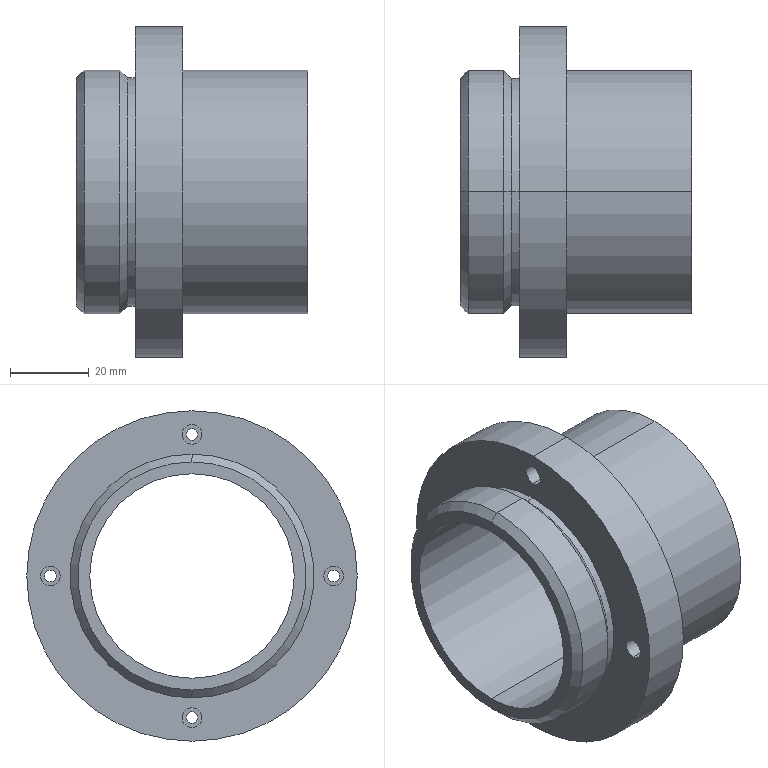Part | SolidWorks | features Chamfer 2, ICE 2, Revolution 1 | 1 solid | 38 faces | box 58.8 x 84 x 84 mm | volume 80812 mm3 | cylinder 26 | plane 8 | cone 4 | commonest cylinder face diameters 3 x8 5 x8 62 x4 52 x2 58 x2 84 x2
STEP:
#1=CARTESIAN_POINT('',(-17.378,0.,33.5));
#2=VERTEX_POINT('',#1);
#3=CARTESIAN_POINT('',(-17.378,0.,38.5));
#4=VERTEX_POINT('',#3);
#5=CARTESIAN_POINT('',(-17.378,0.,36.));
#6=DIRECTION('',(-1.,0.,0.));
#7=DIRECTION('',(0.,0.,1.));
#8=AXIS2_PLACEMENT_3D('',#5,#6,#7);
#9=CIRCLE('',#8,2.5);
#10=EDGE_CURVE('',#2,#4,#9,.T.);
#11=ORIENTED_EDGE('',*,*,#10,.F.);
#12=CARTESIAN_POINT('',(-22.378,0.,33.5));
#13=VERTEX_POINT('',#12);
#14=CARTESIAN_POINT('',(-17.378,0.,33.5));
#15=DIRECTION('',(-1.,0.,0.));
#16=VECTOR('',#15,1000.);
#17=LINE('',#14,#16);
#18=EDGE_CURVE('',#2,#13,#17,.T.);
#19=ORIENTED_EDGE('',*,*,#18,.T.);
#20=CARTESIAN_POINT('',(-22.378,0.,38.5));
#21=VERTEX_POINT('',#20);
#22=CARTESIAN_POINT('',(-22.378,0.,36.));
#23=DIRECTION('',(-1.,0.,0.));
#24=DIRECTION('',(0.,0.,1.));
#25=AXIS2_PLACEMENT_3D('',#22,#23,#24);
#26=CIRCLE('',#25,2.5);
#27=EDGE_CURVE('',#13,#21,#26,.T.);
#28=ORIENTED_EDGE('',*,*,#27,.T.);
#29=CARTESIAN_POINT('',(-17.378,0.,38.5));
#30=DIRECTION('',(-1.,0.,0.));
#31=VECTOR('',#30,1000.);
#32=LINE('',#29,#31);
#33=EDGE_CURVE('',#4,#21,#32,.T.);
#34=ORIENTED_EDGE('',*,*,#33,.F.);
#35=EDGE_LOOP('',(#11,#19,#28,#34));
#36=FACE_OUTER_BOUND('',#35,.T.);
#37=CARTESIAN_POINT('',(-17.378,0.,36.));
#38=DIRECTION('',(-1.,0.,0.));
#39=DIRECTION('',(0.,0.,1.));
#40=AXIS2_PLACEMENT_3D('',#37,#38,#39);
#41=CYLINDRICAL_SURFACE('',#40,2.5);
#42=ADVANCED_FACE('',(#36),#41,.F.);
#43=CARTESIAN_POINT('',(-17.378,36.,-2.5));
#44=VERTEX_POINT('',#43);
#45=CARTESIAN_POINT('',(-17.378,36.,2.5));
#46=VERTEX_POINT('',#45);
#47=CARTESIAN_POINT('',(-17.378,36.,0.));
#48=DIRECTION('',(-1.,0.,0.));
#49=DIRECTION('',(0.,0.,1.));
#50=AXIS2_PLACEMENT_3D('',#47,#48,#49);
#51=CIRCLE('',#50,2.5);
#52=EDGE_CURVE('',#44,#46,#51,.T.);
#53=ORIENTED_EDGE('',*,*,#52,.F.);
#54=CARTESIAN_POINT('',(-22.378,36.,-2.5));
#55=VERTEX_POINT('',#54);
#56=CARTESIAN_POINT('',(-17.378,36.,-2.5));
#57=DIRECTION('',(-1.,0.,0.));
#58=VECTOR('',#57,1000.);
#59=LINE('',#56,#58);
#60=EDGE_CURVE('',#44,#55,#59,.T.);
#61=ORIENTED_EDGE('',*,*,#60,.T.);
#62=CARTESIAN_POINT('',(-22.378,36.,2.5));
#63=VERTEX_POINT('',#62);
#64=CARTESIAN_POINT('',(-22.378,36.,0.));
#65=DIRECTION('',(-1.,0.,0.));
#66=DIRECTION('',(0.,0.,1.));
#67=AXIS2_PLACEMENT_3D('',#64,#65,#66);
#68=CIRCLE('',#67,2.5);
#69=EDGE_CURVE('',#55,#63,#68,.T.);
#70=ORIENTED_EDGE('',*,*,#69,.T.);
#71=CARTESIAN_POINT('',(-17.378,36.,2.5));
#72=DIRECTION('',(-1.,0.,0.));
#73=VECTOR('',#72,1000.);
#74=LINE('',#71,#73);
#75=EDGE_CURVE('',#46,#63,#74,.T.);
#76=ORIENTED_EDGE('',*,*,#75,.F.);
#77=EDGE_LOOP('',(#53,#61,#70,#76));
#78=FACE_OUTER_BOUND('',#77,.T.);
#79=CARTESIAN_POINT('',(-17.378,36.,0.));
#80=DIRECTION('',(-1.,0.,0.));
#81=DIRECTION('',(0.,0.,1.));
#82=AXIS2_PLACEMENT_3D('',#79,#80,#81);
#83=CYLINDRICAL_SURFACE('',#82,2.5);
#84=ADVANCED_FACE('',(#78),#83,.F.);
#85=CARTESIAN_POINT('',(-17.378,0.,-38.5));
#86=VERTEX_POINT('',#85);
#87=CARTESIAN_POINT('',(-17.378,0.,-33.5));
#88=VERTEX_POINT('',#87);
#89=CARTESIAN_POINT('',(-17.378,0.,-36.));
#90=DIRECTION('',(-1.,0.,0.));
#91=DIRECTION('',(0.,0.,1.));
#92=AXIS2_PLACEMENT_3D('',#89,#90,#91);
#93=CIRCLE('',#92,2.5);
#94=EDGE_CURVE('',#86,#88,#93,.T.);
#95=ORIENTED_EDGE('',*,*,#94,.F.);
#96=CARTESIAN_POINT('',(-22.378,0.,-38.5));
#97=VERTEX_POINT('',#96);
#98=CARTESIAN_POINT('',(-17.378,0.,-38.5));
#99=DIRECTION('',(-1.,0.,0.));
#100=VECTOR('',#99,1000.);
#101=LINE('',#98,#100);
#102=EDGE_CURVE('',#86,#97,#101,.T.);
#103=ORIENTED_EDGE('',*,*,#102,.T.);
#104=CARTESIAN_POINT('',(-22.378,0.,-33.5));
#105=VERTEX_POINT('',#104);
#106=CARTESIAN_POINT('',(-22.378,0.,-36.));
#107=DIRECTION('',(-1.,0.,0.));
#108=DIRECTION('',(0.,0.,1.));
#109=AXIS2_PLACEMENT_3D('',#106,#107,#108);
#110=CIRCLE('',#109,2.5);
#111=EDGE_CURVE('',#97,#105,#110,.T.);
#112=ORIENTED_EDGE('',*,*,#111,.T.);
#113=CARTESIAN_POINT('',(-17.378,0.,-33.5));
#114=DIRECTION('',(-1.,0.,0.));
#115=VECTOR('',#114,1000.);
#116=LINE('',#113,#115);
#117=EDGE_CURVE('',#88,#105,#116,.T.);
#118=ORIENTED_EDGE('',*,*,#117,.F.);
#119=EDGE_LOOP('',(#95,#103,#112,#118));
#120=FACE_OUTER_BOUND('',#119,.T.);
#121=CARTESIAN_POINT('',(-17.378,0.,-36.));
#122=DIRECTION('',(-1.,0.,0.));
#123=DIRECTION('',(0.,0.,1.));
#124=AXIS2_PLACEMENT_3D('',#121,#122,#123);
#125=CYLINDRICAL_SURFACE('',#124,2.5);
#126=ADVANCED_FACE('',(#120),#125,.F.);
#127=CARTESIAN_POINT('',(-17.378,-36.,-2.5));
#128=VERTEX_POINT('',#127);
#129=CARTESIAN_POINT('',(-17.378,-36.,2.5));
#130=VERTEX_POINT('',#129);
#131=CARTESIAN_POINT('',(-17.378,-36.,0.));
#132=DIRECTION('',(-1.,0.,0.));
#133=DIRECTION('',(0.,0.,1.));
#134=AXIS2_PLACEMENT_3D('',#131,#132,#133);
#135=CIRCLE('',#134,2.5);
#136=EDGE_CURVE('',#128,#130,#135,.T.);
#137=ORIENTED_EDGE('',*,*,#136,.F.);
#138=CARTESIAN_POINT('',(-22.378,-36.,-2.5));
#139=VERTEX_POINT('',#138);
#140=CARTESIAN_POINT('',(-17.378,-36.,-2.5));
#141=DIRECTION('',(-1.,0.,0.));
#142=VECTOR('',#141,1000.);
#143=LINE('',#140,#142);
#144=EDGE_CURVE('',#128,#139,#143,.T.);
#145=ORIENTED_EDGE('',*,*,#144,.T.);
#146=CARTESIAN_POINT('',(-22.378,-36.,2.5));
#147=VERTEX_POINT('',#146);
#148=CARTESIAN_POINT('',(-22.378,-36.,0.));
#149=DIRECTION('',(-1.,0.,0.));
#150=DIRECTION('',(0.,0.,1.));
#151=AXIS2_PLACEMENT_3D('',#148,#149,#150);
#152=CIRCLE('',#151,2.5);
#153=EDGE_CURVE('',#139,#147,#152,.T.);
#154=ORIENTED_EDGE('',*,*,#153,.T.);
#155=CARTESIAN_POINT('',(-17.378,-36.,2.5));
#156=DIRECTION('',(-1.,0.,0.));
#157=VECTOR('',#156,1000.);
#158=LINE('',#155,#157);
#159=EDGE_CURVE('',#130,#147,#158,.T.);
#160=ORIENTED_EDGE('',*,*,#159,.F.);
#161=EDGE_LOOP('',(#137,#145,#154,#160));
#162=FACE_OUTER_BOUND('',#161,.T.);
#163=CARTESIAN_POINT('',(-17.378,-36.,0.));
#164=DIRECTION('',(-1.,0.,0.));
#165=DIRECTION('',(0.,0.,1.));
#166=AXIS2_PLACEMENT_3D('',#163,#164,#165);
#167=CYLINDRICAL_SURFACE('',#166,2.5);
#168=ADVANCED_FACE('',(#162),#167,.F.);
#169=CARTESIAN_POINT('',(-24.378,0.,29.));
#170=VERTEX_POINT('',#169);
#171=CARTESIAN_POINT('',(-24.378,0.,-29.));
#172=VERTEX_POINT('',#171);
#173=CARTESIAN_POINT('',(-24.378,0.,0.));
#174=DIRECTION('',(-1.,0.,0.));
#175=DIRECTION('',(0.,0.,1.));
#176=AXIS2_PLACEMENT_3D('',#173,#174,#175);
#177=CIRCLE('',#176,29.);
#178=EDGE_CURVE('',#170,#172,#177,.T.);
#179=ORIENTED_EDGE('',*,*,#178,.T.);
#180=CARTESIAN_POINT('',(-26.378,0.,-31.));
#181=VERTEX_POINT('',#180);
#182=CARTESIAN_POINT('',(-26.378,0.,-31.));
#183=DIRECTION('',(-0.7071,0.,-0.7071));
#184=VECTOR('',#183,1000.);
#185=LINE('',#182,#184);
#186=EDGE_CURVE('',#172,#181,#185,.T.);
#187=ORIENTED_EDGE('',*,*,#186,.T.);
#188=CARTESIAN_POINT('',(-26.378,0.,31.));
#189=VERTEX_POINT('',#188);
#190=CARTESIAN_POINT('',(-26.378,0.,0.));
#191=DIRECTION('',(-1.,0.,0.));
#192=DIRECTION('',(0.,0.,1.));
#193=AXIS2_PLACEMENT_3D('',#190,#191,#192);
#194=CIRCLE('',#193,31.);
#195=EDGE_CURVE('',#189,#181,#194,.T.);
#196=ORIENTED_EDGE('',*,*,#195,.F.);
#197=CARTESIAN_POINT('',(-26.378,0.,31.));
#198=DIRECTION('',(-0.7071,0.,0.7071));
#199=VECTOR('',#198,1000.);
#200=LINE('',#197,#199);
#201=EDGE_CURVE('',#170,#189,#200,.T.);
#202=ORIENTED_EDGE('',*,*,#201,.F.);
#203=EDGE_LOOP('',(#179,#187,#196,#202));
#204=FACE_OUTER_BOUND('',#203,.T.);
#205=CARTESIAN_POINT('',(-26.378,0.,0.));
#206=DIRECTION('',(-1.,0.,0.));
#207=DIRECTION('',(0.,0.,1.));
#208=AXIS2_PLACEMENT_3D('',#205,#206,#207);
#209=CONICAL_SURFACE('',#208,31.,0.7854);
#210=ADVANCED_FACE('',(#204),#209,.T.);
#211=CARTESIAN_POINT('',(-37.378,0.,29.));
#212=VERTEX_POINT('',#211);
#213=CARTESIAN_POINT('',(-37.378,0.,-29.));
#214=VERTEX_POINT('',#213);
#215=CARTESIAN_POINT('',(-37.378,0.,0.));
#216=DIRECTION('',(-1.,0.,0.));
#217=DIRECTION('',(0.,0.,-1.));
#218=AXIS2_PLACEMENT_3D('',#215,#216,#217);
#219=CIRCLE('',#218,29.);
#220=EDGE_CURVE('',#212,#214,#219,.T.);
#221=ORIENTED_EDGE('',*,*,#220,.F.);
#222=CARTESIAN_POINT('',(-35.378,0.,31.));
#223=VERTEX_POINT('',#222);
#224=CARTESIAN_POINT('',(-37.378,0.,29.));
#225=DIRECTION('',(0.7071,0.,0.7071));
#226=VECTOR('',#225,1000.);
#227=LINE('',#224,#226);
#228=EDGE_CURVE('',#212,#223,#227,.T.);
#229=ORIENTED_EDGE('',*,*,#228,.T.);
#230=CARTESIAN_POINT('',(-35.378,0.,-31.));
#231=VERTEX_POINT('',#230);
#232=CARTESIAN_POINT('',(-35.378,0.,0.));
#233=DIRECTION('',(1.,0.,0.));
#234=DIRECTION('',(0.,0.,-1.));
#235=AXIS2_PLACEMENT_3D('',#232,#233,#234);
#236=CIRCLE('',#235,31.);
#237=EDGE_CURVE('',#231,#223,#236,.T.);
#238=ORIENTED_EDGE('',*,*,#237,.F.);
#239=CARTESIAN_POINT('',(-37.378,0.,-29.));
#240=DIRECTION('',(0.7071,0.,-0.7071));
#241=VECTOR('',#240,1000.);
#242=LINE('',#239,#241);
#243=EDGE_CURVE('',#214,#231,#242,.T.);
#244=ORIENTED_EDGE('',*,*,#243,.F.);
#245=EDGE_LOOP('',(#221,#229,#238,#244));
#246=FACE_OUTER_BOUND('',#245,.T.);
#247=CARTESIAN_POINT('',(-37.378,0.,0.));
#248=DIRECTION('',(1.,0.,0.));
#249=DIRECTION('',(0.,0.,-1.));
#250=AXIS2_PLACEMENT_3D('',#247,#248,#249);
#251=CONICAL_SURFACE('',#250,29.,0.7854);
#252=ADVANCED_FACE('',(#246),#251,.T.);
#253=CARTESIAN_POINT('',(21.422,0.,31.));
#254=VERTEX_POINT('',#253);
#255=CARTESIAN_POINT('',(21.422,0.,-31.));
#256=VERTEX_POINT('',#255);
#257=CARTESIAN_POINT('',(21.422,0.,0.));
#258=DIRECTION('',(-1.,0.,0.));
#259=DIRECTION('',(0.,0.,1.));
#260=AXIS2_PLACEMENT_3D('',#257,#258,#259);
#261=CIRCLE('',#260,31.);
#262=EDGE_CURVE('',#254,#256,#261,.T.);
#263=ORIENTED_EDGE('',*,*,#262,.T.);
#264=CARTESIAN_POINT('',(-10.378,0.,-31.));
#265=VERTEX_POINT('',#264);
#266=CARTESIAN_POINT('',(-47.158,0.,-31.));
#267=DIRECTION('',(-1.,0.,0.));
#268=VECTOR('',#267,1000.);
#269=LINE('',#266,#268);
#270=EDGE_CURVE('',#256,#265,#269,.T.);
#271=ORIENTED_EDGE('',*,*,#270,.T.);
#272=CARTESIAN_POINT('',(-10.378,0.,31.));
#273=VERTEX_POINT('',#272);
#274=CARTESIAN_POINT('',(-10.378,0.,0.));
#275=DIRECTION('',(-1.,0.,0.));
#276=DIRECTION('',(0.,0.,1.));
#277=AXIS2_PLACEMENT_3D('',#274,#275,#276);
#278=CIRCLE('',#277,31.);
#279=EDGE_CURVE('',#273,#265,#278,.T.);
#280=ORIENTED_EDGE('',*,*,#279,.F.);
#281=CARTESIAN_POINT('',(-47.158,0.,31.));
#282=DIRECTION('',(-1.,0.,0.));
#283=VECTOR('',#282,1000.);
#284=LINE('',#281,#283);
#285=EDGE_CURVE('',#254,#273,#284,.T.);
#286=ORIENTED_EDGE('',*,*,#285,.F.);
#287=EDGE_LOOP('',(#263,#271,#280,#286));
#288=FACE_OUTER_BOUND('',#287,.T.);
#289=CARTESIAN_POINT('',(-47.158,0.,0.));
#290=DIRECTION('',(-1.,0.,0.));
#291=DIRECTION('',(0.,0.,1.));
#292=AXIS2_PLACEMENT_3D('',#289,#290,#291);
#293=CYLINDRICAL_SURFACE('',#292,31.);
#294=ADVANCED_FACE('',(#288),#293,.T.);
#295=CARTESIAN_POINT('',(-10.378,0.,42.));
#296=VERTEX_POINT('',#295);
#297=CARTESIAN_POINT('',(-10.378,0.,-42.));
#298=VERTEX_POINT('',#297);
#299=CARTESIAN_POINT('',(-10.378,0.,0.));
#300=DIRECTION('',(-1.,0.,0.));
#301=DIRECTION('',(0.,0.,1.));
#302=AXIS2_PLACEMENT_3D('',#299,#300,#301);
#303=CIRCLE('',#302,42.);
#304=EDGE_CURVE('',#296,#298,#303,.T.);
#305=ORIENTED_EDGE('',*,*,#304,.T.);
#306=CARTESIAN_POINT('',(-22.378,0.,-42.));
#307=VERTEX_POINT('',#306);
#308=CARTESIAN_POINT('',(-47.158,0.,-42.));
#309=DIRECTION('',(-1.,0.,0.));
#310=VECTOR('',#309,1000.);
#311=LINE('',#308,#310);
#312=EDGE_CURVE('',#298,#307,#311,.T.);
#313=ORIENTED_EDGE('',*,*,#312,.T.);
#314=CARTESIAN_POINT('',(-22.378,0.,42.));
#315=VERTEX_POINT('',#314);
#316=CARTESIAN_POINT('',(-22.378,0.,0.));
#317=DIRECTION('',(-1.,0.,0.));
#318=DIRECTION('',(0.,0.,1.));
#319=AXIS2_PLACEMENT_3D('',#316,#317,#318);
#320=CIRCLE('',#319,42.);
#321=EDGE_CURVE('',#315,#307,#320,.T.);
#322=ORIENTED_EDGE('',*,*,#321,.F.);
#323=CARTESIAN_POINT('',(-47.158,0.,42.));
#324=DIRECTION('',(-1.,0.,0.));
#325=VECTOR('',#324,1000.);
#326=LINE('',#323,#325);
#327=EDGE_CURVE('',#296,#315,#326,.T.);
#328=ORIENTED_EDGE('',*,*,#327,.F.);
#329=EDGE_LOOP('',(#305,#313,#322,#328));
#330=FACE_OUTER_BOUND('',#329,.T.);
#331=CARTESIAN_POINT('',(-47.158,0.,0.));
#332=DIRECTION('',(-1.,0.,0.));
#333=DIRECTION('',(0.,0.,1.));
#334=AXIS2_PLACEMENT_3D('',#331,#332,#333);
#335=CYLINDRICAL_SURFACE('',#334,42.);
#336=ADVANCED_FACE('',(#330),#335,.T.);
#337=CARTESIAN_POINT('',(-22.378,0.,29.));
#338=VERTEX_POINT('',#337);
#339=CARTESIAN_POINT('',(-22.378,0.,-29.));
#340=VERTEX_POINT('',#339);
#341=CARTESIAN_POINT('',(-22.378,0.,0.));
#342=DIRECTION('',(-1.,0.,0.));
#343=DIRECTION('',(0.,0.,1.));
#344=AXIS2_PLACEMENT_3D('',#341,#342,#343);
#345=CIRCLE('',#344,29.);
#346=EDGE_CURVE('',#338,#340,#345,.T.);
#347=ORIENTED_EDGE('',*,*,#346,.T.);
#348=CARTESIAN_POINT('',(-47.158,0.,-29.));
#349=DIRECTION('',(-1.,0.,0.));
#350=VECTOR('',#349,1000.);
#351=LINE('',#348,#350);
#352=EDGE_CURVE('',#340,#172,#351,.T.);
#353=ORIENTED_EDGE('',*,*,#352,.T.);
#354=ORIENTED_EDGE('',*,*,#178,.F.);
#355=CARTESIAN_POINT('',(-47.158,0.,29.));
#356=DIRECTION('',(-1.,0.,0.));
#357=VECTOR('',#356,1000.);
#358=LINE('',#355,#357);
#359=EDGE_CURVE('',#338,#170,#358,.T.);
#360=ORIENTED_EDGE('',*,*,#359,.F.);
#361=EDGE_LOOP('',(#347,#353,#354,#360));
#362=FACE_OUTER_BOUND('',#361,.T.);
#363=CARTESIAN_POINT('',(-47.158,0.,0.));
#364=DIRECTION('',(-1.,0.,0.));
#365=DIRECTION('',(0.,0.,1.));
#366=AXIS2_PLACEMENT_3D('',#363,#364,#365);
#367=CYLINDRICAL_SURFACE('',#366,29.);
#368=ADVANCED_FACE('',(#362),#367,.T.);
#369=ORIENTED_EDGE('',*,*,#195,.T.);
#370=CARTESIAN_POINT('',(-47.158,0.,-31.));
#371=DIRECTION('',(-1.,0.,0.));
#372=VECTOR('',#371,1000.);
#373=LINE('',#370,#372);
#374=EDGE_CURVE('',#181,#231,#373,.T.);
#375=ORIENTED_EDGE('',*,*,#374,.T.);
#376=ORIENTED_EDGE('',*,*,#237,.T.);
#377=CARTESIAN_POINT('',(-47.158,0.,31.));
#378=DIRECTION('',(-1.,0.,0.));
#379=VECTOR('',#378,1000.);
#380=LINE('',#377,#379);
#381=EDGE_CURVE('',#189,#223,#380,.T.);
#382=ORIENTED_EDGE('',*,*,#381,.F.);
#383=EDGE_LOOP('',(#369,#375,#376,#382));
#384=FACE_OUTER_BOUND('',#383,.T.);
#385=CARTESIAN_POINT('',(-47.158,0.,0.));
#386=DIRECTION('',(-1.,0.,0.));
#387=DIRECTION('',(0.,0.,1.));
#388=AXIS2_PLACEMENT_3D('',#385,#386,#387);
#389=CYLINDRICAL_SURFACE('',#388,31.);
#390=ADVANCED_FACE('',(#384),#389,.T.);
#391=CARTESIAN_POINT('',(21.422,0.,-26.));
#392=VERTEX_POINT('',#391);
#393=CARTESIAN_POINT('',(21.422,0.,26.));
#394=VERTEX_POINT('',#393);
#395=CARTESIAN_POINT('',(21.422,0.,0.));
#396=DIRECTION('',(-1.,0.,0.));
#397=DIRECTION('',(0.,0.,1.));
#398=AXIS2_PLACEMENT_3D('',#395,#396,#397);
#399=CIRCLE('',#398,26.);
#400=EDGE_CURVE('',#392,#394,#399,.T.);
#401=ORIENTED_EDGE('',*,*,#400,.F.);
#402=CARTESIAN_POINT('',(-37.378,0.,-26.));
#403=VERTEX_POINT('',#402);
#404=CARTESIAN_POINT('',(-47.158,0.,-26.));
#405=DIRECTION('',(-1.,0.,0.));
#406=VECTOR('',#405,1000.);
#407=LINE('',#404,#406);
#408=EDGE_CURVE('',#392,#403,#407,.T.);
#409=ORIENTED_EDGE('',*,*,#408,.T.);
#410=CARTESIAN_POINT('',(-37.378,0.,26.));
#411=VERTEX_POINT('',#410);
#412=CARTESIAN_POINT('',(-37.378,0.,0.));
#413=DIRECTION('',(-1.,0.,0.));
#414=DIRECTION('',(0.,0.,1.));
#415=AXIS2_PLACEMENT_3D('',#412,#413,#414);
#416=CIRCLE('',#415,26.);
#417=EDGE_CURVE('',#403,#411,#416,.T.);
#418=ORIENTED_EDGE('',*,*,#417,.T.);
#419=CARTESIAN_POINT('',(-47.158,0.,26.));
#420=DIRECTION('',(-1.,0.,0.));
#421=VECTOR('',#420,1000.);
#422=LINE('',#419,#421);
#423=EDGE_CURVE('',#394,#411,#422,.T.);
#424=ORIENTED_EDGE('',*,*,#423,.F.);
#425=EDGE_LOOP('',(#401,#409,#418,#424));
#426=FACE_OUTER_BOUND('',#425,.T.);
#427=CARTESIAN_POINT('',(-47.158,0.,0.));
#428=DIRECTION('',(-1.,0.,0.));
#429=DIRECTION('',(0.,0.,1.));
#430=AXIS2_PLACEMENT_3D('',#427,#428,#429);
#431=CYLINDRICAL_SURFACE('',#430,26.);
#432=ADVANCED_FACE('',(#426),#431,.F.);
#433=CARTESIAN_POINT('',(-10.378,-36.,-1.5));
#434=VERTEX_POINT('',#433);
#435=CARTESIAN_POINT('',(-10.378,-36.,1.5));
#436=VERTEX_POINT('',#435);
#437=CARTESIAN_POINT('',(-10.378,-36.,0.));
#438=DIRECTION('',(-1.,0.,0.));
#439=DIRECTION('',(0.,0.,1.));
#440=AXIS2_PLACEMENT_3D('',#437,#438,#439);
#441=CIRCLE('',#440,1.5);
#442=EDGE_CURVE('',#434,#436,#441,.T.);
#443=ORIENTED_EDGE('',*,*,#442,.F.);
#444=CARTESIAN_POINT('',(-17.378,-36.,-1.5));
#445=VERTEX_POINT('',#444);
#446=CARTESIAN_POINT('',(6.622,-36.,-1.5));
#447=DIRECTION('',(-1.,0.,0.));
#448=VECTOR('',#447,1000.);
#449=LINE('',#446,#448);
#450=EDGE_CURVE('',#434,#445,#449,.T.);
#451=ORIENTED_EDGE('',*,*,#450,.T.);
#452=CARTESIAN_POINT('',(-17.378,-36.,1.5));
#453=VERTEX_POINT('',#452);
#454=CARTESIAN_POINT('',(-17.378,-36.,0.));
#455=DIRECTION('',(1.,0.,0.));
#456=DIRECTION('',(0.,0.,1.));
#457=AXIS2_PLACEMENT_3D('',#454,#455,#456);
#458=CIRCLE('',#457,1.5);
#459=EDGE_CURVE('',#453,#445,#458,.T.);
#460=ORIENTED_EDGE('',*,*,#459,.F.);
#461=CARTESIAN_POINT('',(6.622,-36.,1.5));
#462=DIRECTION('',(-1.,0.,0.));
#463=VECTOR('',#462,1000.);
#464=LINE('',#461,#463);
#465=EDGE_CURVE('',#436,#453,#464,.T.);
#466=ORIENTED_EDGE('',*,*,#465,.F.);
#467=EDGE_LOOP('',(#443,#451,#460,#466));
#468=FACE_OUTER_BOUND('',#467,.T.);
#469=CARTESIAN_POINT('',(6.622,-36.,0.));
#470=DIRECTION('',(-1.,0.,0.));
#471=DIRECTION('',(0.,0.,1.));
#472=AXIS2_PLACEMENT_3D('',#469,#470,#471);
#473=CYLINDRICAL_SURFACE('',#472,1.5);
#474=ADVANCED_FACE('',(#468),#473,.F.);
#475=CARTESIAN_POINT('',(-10.378,0.,-37.5));
#476=VERTEX_POINT('',#475);
#477=CARTESIAN_POINT('',(-10.378,0.,-34.5));
#478=VERTEX_POINT('',#477);
#479=CARTESIAN_POINT('',(-10.378,0.,-36.));
#480=DIRECTION('',(-1.,0.,0.));
#481=DIRECTION('',(0.,0.,1.));
#482=AXIS2_PLACEMENT_3D('',#479,#480,#481);
#483=CIRCLE('',#482,1.5);
#484=EDGE_CURVE('',#476,#478,#483,.T.);
#485=ORIENTED_EDGE('',*,*,#484,.F.);
#486=CARTESIAN_POINT('',(-17.378,0.,-37.5));
#487=VERTEX_POINT('',#486);
#488=CARTESIAN_POINT('',(6.622,0.,-37.5));
#489=DIRECTION('',(-1.,0.,0.));
#490=VECTOR('',#489,1000.);
#491=LINE('',#488,#490);
#492=EDGE_CURVE('',#476,#487,#491,.T.);
#493=ORIENTED_EDGE('',*,*,#492,.T.);
#494=CARTESIAN_POINT('',(-17.378,0.,-34.5));
#495=VERTEX_POINT('',#494);
#496=CARTESIAN_POINT('',(-17.378,0.,-36.));
#497=DIRECTION('',(1.,0.,0.));
#498=DIRECTION('',(0.,0.,1.));
#499=AXIS2_PLACEMENT_3D('',#496,#497,#498);
#500=CIRCLE('',#499,1.5);
#501=EDGE_CURVE('',#495,#487,#500,.T.);
#502=ORIENTED_EDGE('',*,*,#501,.F.);
#503=CARTESIAN_POINT('',(6.622,0.,-34.5));
#504=DIRECTION('',(-1.,0.,0.));
#505=VECTOR('',#504,1000.);
#506=LINE('',#503,#505);
#507=EDGE_CURVE('',#478,#495,#506,.T.);
#508=ORIENTED_EDGE('',*,*,#507,.F.);
#509=EDGE_LOOP('',(#485,#493,#502,#508));
#510=FACE_OUTER_BOUND('',#509,.T.);
#511=CARTESIAN_POINT('',(6.622,0.,-36.));
#512=DIRECTION('',(-1.,0.,0.));
#513=DIRECTION('',(0.,0.,1.));
#514=AXIS2_PLACEMENT_3D('',#511,#512,#513);
#515=CYLINDRICAL_SURFACE('',#514,1.5);
#516=ADVANCED_FACE('',(#510),#515,.F.);
#517=CARTESIAN_POINT('',(-10.378,36.,-1.5));
#518=VERTEX_POINT('',#517);
#519=CARTESIAN_POINT('',(-10.378,36.,1.5));
#520=VERTEX_POINT('',#519);
#521=CARTESIAN_POINT('',(-10.378,36.,0.));
#522=DIRECTION('',(-1.,0.,0.));
#523=DIRECTION('',(0.,0.,1.));
#524=AXIS2_PLACEMENT_3D('',#521,#522,#523);
#525=CIRCLE('',#524,1.5);
#526=EDGE_CURVE('',#518,#520,#525,.T.);
#527=ORIENTED_EDGE('',*,*,#526,.F.);
#528=CARTESIAN_POINT('',(-17.378,36.,-1.5));
#529=VERTEX_POINT('',#528);
#530=CARTESIAN_POINT('',(6.622,36.,-1.5));
#531=DIRECTION('',(-1.,0.,0.));
#532=VECTOR('',#531,1000.);
#533=LINE('',#530,#532);
#534=EDGE_CURVE('',#518,#529,#533,.T.);
#535=ORIENTED_EDGE('',*,*,#534,.T.);
#536=CARTESIAN_POINT('',(-17.378,36.,1.5));
#537=VERTEX_POINT('',#536);
#538=CARTESIAN_POINT('',(-17.378,36.,0.));
#539=DIRECTION('',(1.,0.,0.));
#540=DIRECTION('',(0.,0.,1.));
#541=AXIS2_PLACEMENT_3D('',#538,#539,#540);
#542=CIRCLE('',#541,1.5);
#543=EDGE_CURVE('',#537,#529,#542,.T.);
#544=ORIENTED_EDGE('',*,*,#543,.F.);
#545=CARTESIAN_POINT('',(6.622,36.,1.5));
#546=DIRECTION('',(-1.,0.,0.));
#547=VECTOR('',#546,1000.);
#548=LINE('',#545,#547);
#549=EDGE_CURVE('',#520,#537,#548,.T.);
#550=ORIENTED_EDGE('',*,*,#549,.F.);
#551=EDGE_LOOP('',(#527,#535,#544,#550));
#552=FACE_OUTER_BOUND('',#551,.T.);
#553=CARTESIAN_POINT('',(6.622,36.,0.));
#554=DIRECTION('',(-1.,0.,0.));
#555=DIRECTION('',(0.,0.,1.));
#556=AXIS2_PLACEMENT_3D('',#553,#554,#555);
#557=CYLINDRICAL_SURFACE('',#556,1.5);
#558=ADVANCED_FACE('',(#552),#557,.F.);
#559=CARTESIAN_POINT('',(-10.378,0.,34.5));
#560=VERTEX_POINT('',#559);
#561=CARTESIAN_POINT('',(-10.378,0.,37.5));
#562=VERTEX_POINT('',#561);
#563=CARTESIAN_POINT('',(-10.378,0.,36.));
#564=DIRECTION('',(-1.,0.,0.));
#565=DIRECTION('',(0.,0.,1.));
#566=AXIS2_PLACEMENT_3D('',#563,#564,#565);
#567=CIRCLE('',#566,1.5);
#568=EDGE_CURVE('',#560,#562,#567,.T.);
#569=ORIENTED_EDGE('',*,*,#568,.F.);
#570=CARTESIAN_POINT('',(-17.378,0.,34.5));
#571=VERTEX_POINT('',#570);
#572=CARTESIAN_POINT('',(6.622,0.,34.5));
#573=DIRECTION('',(-1.,0.,0.));
#574=VECTOR('',#573,1000.);
#575=LINE('',#572,#574);
#576=EDGE_CURVE('',#560,#571,#575,.T.);
#577=ORIENTED_EDGE('',*,*,#576,.T.);
#578=CARTESIAN_POINT('',(-17.378,0.,37.5));
#579=VERTEX_POINT('',#578);
#580=CARTESIAN_POINT('',(-17.378,0.,36.));
#581=DIRECTION('',(1.,0.,0.));
#582=DIRECTION('',(0.,0.,1.));
#583=AXIS2_PLACEMENT_3D('',#580,#581,#582);
#584=CIRCLE('',#583,1.5);
#585=EDGE_CURVE('',#579,#571,#584,.T.);
#586=ORIENTED_EDGE('',*,*,#585,.F.);
#587=CARTESIAN_POINT('',(6.622,0.,37.5));
#588=DIRECTION('',(-1.,0.,0.));
#589=VECTOR('',#588,1000.);
#590=LINE('',#587,#589);
#591=EDGE_CURVE('',#562,#579,#590,.T.);
#592=ORIENTED_EDGE('',*,*,#591,.F.);
#593=EDGE_LOOP('',(#569,#577,#586,#592));
#594=FACE_OUTER_BOUND('',#593,.T.);
#595=CARTESIAN_POINT('',(6.622,0.,36.));
#596=DIRECTION('',(-1.,0.,0.));
#597=DIRECTION('',(0.,0.,1.));
#598=AXIS2_PLACEMENT_3D('',#595,#596,#597);
#599=CYLINDRICAL_SURFACE('',#598,1.5);
#600=ADVANCED_FACE('',(#594),#599,.F.);
#601=ORIENTED_EDGE('',*,*,#576,.F.);
#602=CARTESIAN_POINT('',(-10.378,0.,36.));
#603=DIRECTION('',(-1.,0.,0.));
#604=DIRECTION('',(0.,0.,1.));
#605=AXIS2_PLACEMENT_3D('',#602,#603,#604);
#606=CIRCLE('',#605,1.5);
#607=EDGE_CURVE('',#562,#560,#606,.T.);
#608=ORIENTED_EDGE('',*,*,#607,.F.);
#609=ORIENTED_EDGE('',*,*,#591,.T.);
#610=CARTESIAN_POINT('',(-17.378,0.,36.));
#611=DIRECTION('',(1.,0.,0.));
#612=DIRECTION('',(0.,0.,1.));
#613=AXIS2_PLACEMENT_3D('',#610,#611,#612);
#614=CIRCLE('',#613,1.5);
#615=EDGE_CURVE('',#571,#579,#614,.T.);
#616=ORIENTED_EDGE('',*,*,#615,.F.);
#617=EDGE_LOOP('',(#601,#608,#609,#616));
#618=FACE_OUTER_BOUND('',#617,.T.);
#619=CARTESIAN_POINT('',(6.622,0.,36.));
#620=DIRECTION('',(-1.,0.,0.));
#621=DIRECTION('',(0.,0.,1.));
#622=AXIS2_PLACEMENT_3D('',#619,#620,#621);
#623=CYLINDRICAL_SURFACE('',#622,1.5);
#624=ADVANCED_FACE('',(#618),#623,.F.);
#625=ORIENTED_EDGE('',*,*,#534,.F.);
#626=CARTESIAN_POINT('',(-10.378,36.,0.));
#627=DIRECTION('',(-1.,0.,0.));
#628=DIRECTION('',(0.,0.,1.));
#629=AXIS2_PLACEMENT_3D('',#626,#627,#628);
#630=CIRCLE('',#629,1.5);
#631=EDGE_CURVE('',#520,#518,#630,.T.);
#632=ORIENTED_EDGE('',*,*,#631,.F.);
#633=ORIENTED_EDGE('',*,*,#549,.T.);
#634=CARTESIAN_POINT('',(-17.378,36.,0.));
#635=DIRECTION('',(1.,0.,0.));
#636=DIRECTION('',(0.,0.,1.));
#637=AXIS2_PLACEMENT_3D('',#634,#635,#636);
#638=CIRCLE('',#637,1.5);
#639=EDGE_CURVE('',#529,#537,#638,.T.);
#640=ORIENTED_EDGE('',*,*,#639,.F.);
#641=EDGE_LOOP('',(#625,#632,#633,#640));
#642=FACE_OUTER_BOUND('',#641,.T.);
#643=CARTESIAN_POINT('',(6.622,36.,0.));
#644=DIRECTION('',(-1.,0.,0.));
#645=DIRECTION('',(0.,0.,1.));
#646=AXIS2_PLACEMENT_3D('',#643,#644,#645);
#647=CYLINDRICAL_SURFACE('',#646,1.5);
#648=ADVANCED_FACE('',(#642),#647,.F.);
#649=ORIENTED_EDGE('',*,*,#492,.F.);
#650=CARTESIAN_POINT('',(-10.378,0.,-36.));
#651=DIRECTION('',(-1.,0.,0.));
#652=DIRECTION('',(0.,0.,1.));
#653=AXIS2_PLACEMENT_3D('',#650,#651,#652);
#654=CIRCLE('',#653,1.5);
#655=EDGE_CURVE('',#478,#476,#654,.T.);
#656=ORIENTED_EDGE('',*,*,#655,.F.);
#657=ORIENTED_EDGE('',*,*,#507,.T.);
#658=CARTESIAN_POINT('',(-17.378,0.,-36.));
#659=DIRECTION('',(1.,0.,0.));
#660=DIRECTION('',(0.,0.,1.));
#661=AXIS2_PLACEMENT_3D('',#658,#659,#660);
#662=CIRCLE('',#661,1.5);
#663=EDGE_CURVE('',#487,#495,#662,.T.);
#664=ORIENTED_EDGE('',*,*,#663,.F.);
#665=EDGE_LOOP('',(#649,#656,#657,#664));
#666=FACE_OUTER_BOUND('',#665,.T.);
#667=CARTESIAN_POINT('',(6.622,0.,-36.));
#668=DIRECTION('',(-1.,0.,0.));
#669=DIRECTION('',(0.,0.,1.));
#670=AXIS2_PLACEMENT_3D('',#667,#668,#669);
#671=CYLINDRICAL_SURFACE('',#670,1.5);
#672=ADVANCED_FACE('',(#666),#671,.F.);
#673=ORIENTED_EDGE('',*,*,#450,.F.);
#674=CARTESIAN_POINT('',(-10.378,-36.,0.));
#675=DIRECTION('',(-1.,0.,0.));
#676=DIRECTION('',(0.,0.,1.));
#677=AXIS2_PLACEMENT_3D('',#674,#675,#676);
#678=CIRCLE('',#677,1.5);
#679=EDGE_CURVE('',#436,#434,#678,.T.);
#680=ORIENTED_EDGE('',*,*,#679,.F.);
#681=ORIENTED_EDGE('',*,*,#465,.T.);
#682=CARTESIAN_POINT('',(-17.378,-36.,0.));
#683=DIRECTION('',(1.,0.,0.));
#684=DIRECTION('',(0.,0.,1.));
#685=AXIS2_PLACEMENT_3D('',#682,#683,#684);
#686=CIRCLE('',#685,1.5);
#687=EDGE_CURVE('',#445,#453,#686,.T.);
#688=ORIENTED_EDGE('',*,*,#687,.F.);
#689=EDGE_LOOP('',(#673,#680,#681,#688));
#690=FACE_OUTER_BOUND('',#689,.T.);
#691=CARTESIAN_POINT('',(6.622,-36.,0.));
#692=DIRECTION('',(-1.,0.,0.));
#693=DIRECTION('',(0.,0.,1.));
#694=AXIS2_PLACEMENT_3D('',#691,#692,#693);
#695=CYLINDRICAL_SURFACE('',#694,1.5);
#696=ADVANCED_FACE('',(#690),#695,.F.);
#697=ORIENTED_EDGE('',*,*,#408,.F.);
#698=CARTESIAN_POINT('',(21.422,0.,0.));
#699=DIRECTION('',(-1.,0.,0.));
#700=DIRECTION('',(0.,0.,1.));
#701=AXIS2_PLACEMENT_3D('',#698,#699,#700);
#702=CIRCLE('',#701,26.);
#703=EDGE_CURVE('',#394,#392,#702,.T.);
#704=ORIENTED_EDGE('',*,*,#703,.F.);
#705=ORIENTED_EDGE('',*,*,#423,.T.);
#706=CARTESIAN_POINT('',(-37.378,0.,0.));
#707=DIRECTION('',(-1.,0.,0.));
#708=DIRECTION('',(0.,0.,1.));
#709=AXIS2_PLACEMENT_3D('',#706,#707,#708);
#710=CIRCLE('',#709,26.);
#711=EDGE_CURVE('',#411,#403,#710,.T.);
#712=ORIENTED_EDGE('',*,*,#711,.T.);
#713=EDGE_LOOP('',(#697,#704,#705,#712));
#714=FACE_OUTER_BOUND('',#713,.T.);
#715=CARTESIAN_POINT('',(-47.158,0.,0.));
#716=DIRECTION('',(-1.,0.,0.));
#717=DIRECTION('',(0.,0.,1.));
#718=AXIS2_PLACEMENT_3D('',#715,#716,#717);
#719=CYLINDRICAL_SURFACE('',#718,26.);
#720=ADVANCED_FACE('',(#714),#719,.F.);
#721=CARTESIAN_POINT('',(-37.378,0.,0.));
#722=DIRECTION('',(-1.,0.,0.));
#723=DIRECTION('',(0.,0.,-1.));
#724=AXIS2_PLACEMENT_3D('',#721,#722,#723);
#725=CIRCLE('',#724,29.);
#726=EDGE_CURVE('',#214,#212,#725,.T.);
#727=ORIENTED_EDGE('',*,*,#726,.T.);
#728=ORIENTED_EDGE('',*,*,#220,.T.);
#729=EDGE_LOOP('',(#727,#728));
#730=FACE_OUTER_BOUND('',#729,.T.);
#731=ORIENTED_EDGE('',*,*,#711,.F.);
#732=ORIENTED_EDGE('',*,*,#417,.F.);
#733=EDGE_LOOP('',(#731,#732));
#734=FACE_BOUND('',#733,.T.);
#735=CARTESIAN_POINT('',(-37.378,26.,0.));
#736=DIRECTION('',(1.,0.,0.));
#737=DIRECTION('',(0.,0.,-1.));
#738=AXIS2_PLACEMENT_3D('',#735,#736,#737);
#739=PLANE('',#738);
#740=ADVANCED_FACE('',(#730,#734),#739,.F.);
#741=ORIENTED_EDGE('',*,*,#374,.F.);
#742=CARTESIAN_POINT('',(-26.378,0.,0.));
#743=DIRECTION('',(-1.,0.,0.));
#744=DIRECTION('',(0.,0.,1.));
#745=AXIS2_PLACEMENT_3D('',#742,#743,#744);
#746=CIRCLE('',#745,31.);
#747=EDGE_CURVE('',#181,#189,#746,.T.);
#748=ORIENTED_EDGE('',*,*,#747,.T.);
#749=ORIENTED_EDGE('',*,*,#381,.T.);
#750=CARTESIAN_POINT('',(-35.378,0.,0.));
#751=DIRECTION('',(1.,0.,0.));
#752=DIRECTION('',(0.,0.,-1.));
#753=AXIS2_PLACEMENT_3D('',#750,#751,#752);
#754=CIRCLE('',#753,31.);
#755=EDGE_CURVE('',#223,#231,#754,.T.);
#756=ORIENTED_EDGE('',*,*,#755,.T.);
#757=EDGE_LOOP('',(#741,#748,#749,#756));
#758=FACE_OUTER_BOUND('',#757,.T.);
#759=CARTESIAN_POINT('',(-47.158,0.,0.));
#760=DIRECTION('',(-1.,0.,0.));
#761=DIRECTION('',(0.,0.,1.));
#762=AXIS2_PLACEMENT_3D('',#759,#760,#761);
#763=CYLINDRICAL_SURFACE('',#762,31.);
#764=ADVANCED_FACE('',(#758),#763,.T.);
#765=ORIENTED_EDGE('',*,*,#352,.F.);
#766=CARTESIAN_POINT('',(-22.378,0.,0.));
#767=DIRECTION('',(-1.,0.,0.));
#768=DIRECTION('',(0.,0.,1.));
#769=AXIS2_PLACEMENT_3D('',#766,#767,#768);
#770=CIRCLE('',#769,29.);
#771=EDGE_CURVE('',#340,#338,#770,.T.);
#772=ORIENTED_EDGE('',*,*,#771,.T.);
#773=ORIENTED_EDGE('',*,*,#359,.T.);
#774=CARTESIAN_POINT('',(-24.378,0.,0.));
#775=DIRECTION('',(-1.,0.,0.));
#776=DIRECTION('',(0.,0.,1.));
#777=AXIS2_PLACEMENT_3D('',#774,#775,#776);
#778=CIRCLE('',#777,29.);
#779=EDGE_CURVE('',#172,#170,#778,.T.);
#780=ORIENTED_EDGE('',*,*,#779,.F.);
#781=EDGE_LOOP('',(#765,#772,#773,#780));
#782=FACE_OUTER_BOUND('',#781,.T.);
#783=CARTESIAN_POINT('',(-47.158,0.,0.));
#784=DIRECTION('',(-1.,0.,0.));
#785=DIRECTION('',(0.,0.,1.));
#786=AXIS2_PLACEMENT_3D('',#783,#784,#785);
#787=CYLINDRICAL_SURFACE('',#786,29.);
#788=ADVANCED_FACE('',(#782),#787,.T.);
#789=CARTESIAN_POINT('',(-22.378,0.,-36.));
#790=DIRECTION('',(-1.,0.,0.));
#791=DIRECTION('',(0.,0.,1.));
#792=AXIS2_PLACEMENT_3D('',#789,#790,#791);
#793=CIRCLE('',#792,2.5);
#794=EDGE_CURVE('',#105,#97,#793,.T.);
#795=ORIENTED_EDGE('',*,*,#794,.F.);
#796=ORIENTED_EDGE('',*,*,#111,.F.);
#797=EDGE_LOOP('',(#795,#796));
#798=FACE_BOUND('',#797,.T.);
#799=CARTESIAN_POINT('',(-22.378,36.,0.));
#800=DIRECTION('',(-1.,0.,0.));
#801=DIRECTION('',(0.,0.,1.));
#802=AXIS2_PLACEMENT_3D('',#799,#800,#801);
#803=CIRCLE('',#802,2.5);
#804=EDGE_CURVE('',#63,#55,#803,.T.);
#805=ORIENTED_EDGE('',*,*,#804,.F.);
#806=ORIENTED_EDGE('',*,*,#69,.F.);
#807=EDGE_LOOP('',(#805,#806));
#808=FACE_BOUND('',#807,.T.);
#809=CARTESIAN_POINT('',(-22.378,0.,36.));
#810=DIRECTION('',(-1.,0.,0.));
#811=DIRECTION('',(0.,0.,1.));
#812=AXIS2_PLACEMENT_3D('',#809,#810,#811);
#813=CIRCLE('',#812,2.5);
#814=EDGE_CURVE('',#21,#13,#813,.T.);
#815=ORIENTED_EDGE('',*,*,#814,.F.);
#816=ORIENTED_EDGE('',*,*,#27,.F.);
#817=EDGE_LOOP('',(#815,#816));
#818=FACE_BOUND('',#817,.T.);
#819=CARTESIAN_POINT('',(-22.378,-36.,0.));
#820=DIRECTION('',(-1.,0.,0.));
#821=DIRECTION('',(0.,0.,1.));
#822=AXIS2_PLACEMENT_3D('',#819,#820,#821);
#823=CIRCLE('',#822,2.5);
#824=EDGE_CURVE('',#147,#139,#823,.T.);
#825=ORIENTED_EDGE('',*,*,#824,.F.);
#826=ORIENTED_EDGE('',*,*,#153,.F.);
#827=EDGE_LOOP('',(#825,#826));
#828=FACE_BOUND('',#827,.T.);
#829=ORIENTED_EDGE('',*,*,#346,.F.);
#830=ORIENTED_EDGE('',*,*,#771,.F.);
#831=EDGE_LOOP('',(#829,#830));
#832=FACE_BOUND('',#831,.T.);
#833=ORIENTED_EDGE('',*,*,#321,.T.);
#834=CARTESIAN_POINT('',(-22.378,0.,0.));
#835=DIRECTION('',(-1.,0.,0.));
#836=DIRECTION('',(0.,0.,1.));
#837=AXIS2_PLACEMENT_3D('',#834,#835,#836);
#838=CIRCLE('',#837,42.);
#839=EDGE_CURVE('',#307,#315,#838,.T.);
#840=ORIENTED_EDGE('',*,*,#839,.T.);
#841=EDGE_LOOP('',(#833,#840));
#842=FACE_OUTER_BOUND('',#841,.T.);
#843=CARTESIAN_POINT('',(-22.378,31.,0.));
#844=DIRECTION('',(1.,0.,0.));
#845=DIRECTION('',(0.,0.,-1.));
#846=AXIS2_PLACEMENT_3D('',#843,#844,#845);
#847=PLANE('',#846);
#848=ADVANCED_FACE('',(#798,#808,#818,#828,#832,#842),#847,.F.);
#849=ORIENTED_EDGE('',*,*,#312,.F.);
#850=CARTESIAN_POINT('',(-10.378,0.,0.));
#851=DIRECTION('',(-1.,0.,0.));
#852=DIRECTION('',(0.,0.,1.));
#853=AXIS2_PLACEMENT_3D('',#850,#851,#852);
#854=CIRCLE('',#853,42.);
#855=EDGE_CURVE('',#298,#296,#854,.T.);
#856=ORIENTED_EDGE('',*,*,#855,.T.);
#857=ORIENTED_EDGE('',*,*,#327,.T.);
#858=ORIENTED_EDGE('',*,*,#839,.F.);
#859=EDGE_LOOP('',(#849,#856,#857,#858));
#860=FACE_OUTER_BOUND('',#859,.T.);
#861=CARTESIAN_POINT('',(-47.158,0.,0.));
#862=DIRECTION('',(-1.,0.,0.));
#863=DIRECTION('',(0.,0.,1.));
#864=AXIS2_PLACEMENT_3D('',#861,#862,#863);
#865=CYLINDRICAL_SURFACE('',#864,42.);
#866=ADVANCED_FACE('',(#860),#865,.T.);
#867=ORIENTED_EDGE('',*,*,#655,.T.);
#868=ORIENTED_EDGE('',*,*,#484,.T.);
#869=EDGE_LOOP('',(#867,#868));
#870=FACE_BOUND('',#869,.T.);
#871=ORIENTED_EDGE('',*,*,#631,.T.);
#872=ORIENTED_EDGE('',*,*,#526,.T.);
#873=EDGE_LOOP('',(#871,#872));
#874=FACE_BOUND('',#873,.T.);
#875=ORIENTED_EDGE('',*,*,#607,.T.);
#876=ORIENTED_EDGE('',*,*,#568,.T.);
#877=EDGE_LOOP('',(#875,#876));
#878=FACE_BOUND('',#877,.T.);
#879=ORIENTED_EDGE('',*,*,#679,.T.);
#880=ORIENTED_EDGE('',*,*,#442,.T.);
#881=EDGE_LOOP('',(#879,#880));
#882=FACE_BOUND('',#881,.T.);
#883=ORIENTED_EDGE('',*,*,#304,.F.);
#884=ORIENTED_EDGE('',*,*,#855,.F.);
#885=EDGE_LOOP('',(#883,#884));
#886=FACE_OUTER_BOUND('',#885,.T.);
#887=ORIENTED_EDGE('',*,*,#279,.T.);
#888=CARTESIAN_POINT('',(-10.378,0.,0.));
#889=DIRECTION('',(-1.,0.,0.));
#890=DIRECTION('',(0.,0.,1.));
#891=AXIS2_PLACEMENT_3D('',#888,#889,#890);
#892=CIRCLE('',#891,31.);
#893=EDGE_CURVE('',#265,#273,#892,.T.);
#894=ORIENTED_EDGE('',*,*,#893,.T.);
#895=EDGE_LOOP('',(#887,#894));
#896=FACE_BOUND('',#895,.T.);
#897=CARTESIAN_POINT('',(-10.378,42.,0.));
#898=DIRECTION('',(-1.,0.,0.));
#899=DIRECTION('',(0.,0.,1.));
#900=AXIS2_PLACEMENT_3D('',#897,#898,#899);
#901=PLANE('',#900);
#902=ADVANCED_FACE('',(#870,#874,#878,#882,#886,#896),#901,.F.);
#903=ORIENTED_EDGE('',*,*,#270,.F.);
#904=CARTESIAN_POINT('',(21.422,0.,0.));
#905=DIRECTION('',(-1.,0.,0.));
#906=DIRECTION('',(0.,0.,1.));
#907=AXIS2_PLACEMENT_3D('',#904,#905,#906);
#908=CIRCLE('',#907,31.);
#909=EDGE_CURVE('',#256,#254,#908,.T.);
#910=ORIENTED_EDGE('',*,*,#909,.T.);
#911=ORIENTED_EDGE('',*,*,#285,.T.);
#912=ORIENTED_EDGE('',*,*,#893,.F.);
#913=EDGE_LOOP('',(#903,#910,#911,#912));
#914=FACE_OUTER_BOUND('',#913,.T.);
#915=CARTESIAN_POINT('',(-47.158,0.,0.));
#916=DIRECTION('',(-1.,0.,0.));
#917=DIRECTION('',(0.,0.,1.));
#918=AXIS2_PLACEMENT_3D('',#915,#916,#917);
#919=CYLINDRICAL_SURFACE('',#918,31.);
#920=ADVANCED_FACE('',(#914),#919,.T.);
#921=ORIENTED_EDGE('',*,*,#262,.F.);
#922=ORIENTED_EDGE('',*,*,#909,.F.);
#923=EDGE_LOOP('',(#921,#922));
#924=FACE_OUTER_BOUND('',#923,.T.);
#925=ORIENTED_EDGE('',*,*,#703,.T.);
#926=ORIENTED_EDGE('',*,*,#400,.T.);
#927=EDGE_LOOP('',(#925,#926));
#928=FACE_BOUND('',#927,.T.);
#929=CARTESIAN_POINT('',(21.422,31.,0.));
#930=DIRECTION('',(-1.,0.,0.));
#931=DIRECTION('',(0.,0.,1.));
#932=AXIS2_PLACEMENT_3D('',#929,#930,#931);
#933=PLANE('',#932);
#934=ADVANCED_FACE('',(#924,#928),#933,.F.);
#935=ORIENTED_EDGE('',*,*,#228,.F.);
#936=ORIENTED_EDGE('',*,*,#726,.F.);
#937=ORIENTED_EDGE('',*,*,#243,.T.);
#938=ORIENTED_EDGE('',*,*,#755,.F.);
#939=EDGE_LOOP('',(#935,#936,#937,#938));
#940=FACE_OUTER_BOUND('',#939,.T.);
#941=CARTESIAN_POINT('',(-37.378,0.,0.));
#942=DIRECTION('',(1.,0.,0.));
#943=DIRECTION('',(0.,0.,-1.));
#944=AXIS2_PLACEMENT_3D('',#941,#942,#943);
#945=CONICAL_SURFACE('',#944,29.,0.7854);
#946=ADVANCED_FACE('',(#940),#945,.T.);
#947=ORIENTED_EDGE('',*,*,#186,.F.);
#948=ORIENTED_EDGE('',*,*,#779,.T.);
#949=ORIENTED_EDGE('',*,*,#201,.T.);
#950=ORIENTED_EDGE('',*,*,#747,.F.);
#951=EDGE_LOOP('',(#947,#948,#949,#950));
#952=FACE_OUTER_BOUND('',#951,.T.);
#953=CARTESIAN_POINT('',(-26.378,0.,0.));
#954=DIRECTION('',(-1.,0.,0.));
#955=DIRECTION('',(0.,0.,1.));
#956=AXIS2_PLACEMENT_3D('',#953,#954,#955);
#957=CONICAL_SURFACE('',#956,31.,0.7854);
#958=ADVANCED_FACE('',(#952),#957,.T.);
#959=CARTESIAN_POINT('',(-17.378,-36.,0.));
#960=DIRECTION('',(-1.,0.,0.));
#961=DIRECTION('',(0.,0.,1.));
#962=AXIS2_PLACEMENT_3D('',#959,#960,#961);
#963=CIRCLE('',#962,2.5);
#964=EDGE_CURVE('',#130,#128,#963,.T.);
#965=ORIENTED_EDGE('',*,*,#964,.T.);
#966=ORIENTED_EDGE('',*,*,#136,.T.);
#967=EDGE_LOOP('',(#965,#966));
#968=FACE_OUTER_BOUND('',#967,.T.);
#969=ORIENTED_EDGE('',*,*,#459,.T.);
#970=ORIENTED_EDGE('',*,*,#687,.T.);
#971=EDGE_LOOP('',(#969,#970));
#972=FACE_BOUND('',#971,.T.);
#973=CARTESIAN_POINT('',(-17.378,-36.,0.));
#974=DIRECTION('',(-1.,0.,0.));
#975=DIRECTION('',(0.,0.,1.));
#976=AXIS2_PLACEMENT_3D('',#973,#974,#975);
#977=PLANE('',#976);
#978=ADVANCED_FACE('',(#968,#972),#977,.T.);
#979=ORIENTED_EDGE('',*,*,#144,.F.);
#980=ORIENTED_EDGE('',*,*,#964,.F.);
#981=ORIENTED_EDGE('',*,*,#159,.T.);
#982=ORIENTED_EDGE('',*,*,#824,.T.);
#983=EDGE_LOOP('',(#979,#980,#981,#982));
#984=FACE_OUTER_BOUND('',#983,.T.);
#985=CARTESIAN_POINT('',(-17.378,-36.,0.));
#986=DIRECTION('',(-1.,0.,0.));
#987=DIRECTION('',(0.,0.,1.));
#988=AXIS2_PLACEMENT_3D('',#985,#986,#987);
#989=CYLINDRICAL_SURFACE('',#988,2.5);
#990=ADVANCED_FACE('',(#984),#989,.F.);
#991=CARTESIAN_POINT('',(-17.378,0.,-36.));
#992=DIRECTION('',(-1.,0.,0.));
#993=DIRECTION('',(0.,0.,1.));
#994=AXIS2_PLACEMENT_3D('',#991,#992,#993);
#995=CIRCLE('',#994,2.5);
#996=EDGE_CURVE('',#88,#86,#995,.T.);
#997=ORIENTED_EDGE('',*,*,#996,.T.);
#998=ORIENTED_EDGE('',*,*,#94,.T.);
#999=EDGE_LOOP('',(#997,#998));
#1000=FACE_OUTER_BOUND('',#999,.T.);
#1001=ORIENTED_EDGE('',*,*,#501,.T.);
#1002=ORIENTED_EDGE('',*,*,#663,.T.);
#1003=EDGE_LOOP('',(#1001,#1002));
#1004=FACE_BOUND('',#1003,.T.);
#1005=CARTESIAN_POINT('',(-17.378,0.,-36.));
#1006=DIRECTION('',(-1.,0.,0.));
#1007=DIRECTION('',(0.,0.,1.));
#1008=AXIS2_PLACEMENT_3D('',#1005,#1006,#1007);
#1009=PLANE('',#1008);
#1010=ADVANCED_FACE('',(#1000,#1004),#1009,.T.);
#1011=ORIENTED_EDGE('',*,*,#102,.F.);
#1012=ORIENTED_EDGE('',*,*,#996,.F.);
#1013=ORIENTED_EDGE('',*,*,#117,.T.);
#1014=ORIENTED_EDGE('',*,*,#794,.T.);
#1015=EDGE_LOOP('',(#1011,#1012,#1013,#1014));
#1016=FACE_OUTER_BOUND('',#1015,.T.);
#1017=CARTESIAN_POINT('',(-17.378,0.,-36.));
#1018=DIRECTION('',(-1.,0.,0.));
#1019=DIRECTION('',(0.,0.,1.));
#1020=AXIS2_PLACEMENT_3D('',#1017,#1018,#1019);
#1021=CYLINDRICAL_SURFACE('',#1020,2.5);
#1022=ADVANCED_FACE('',(#1016),#1021,.F.);
#1023=CARTESIAN_POINT('',(-17.378,36.,0.));
#1024=DIRECTION('',(-1.,0.,0.));
#1025=DIRECTION('',(0.,0.,1.));
#1026=AXIS2_PLACEMENT_3D('',#1023,#1024,#1025);
#1027=CIRCLE('',#1026,2.5);
#1028=EDGE_CURVE('',#46,#44,#1027,.T.);
#1029=ORIENTED_EDGE('',*,*,#1028,.T.);
#1030=ORIENTED_EDGE('',*,*,#52,.T.);
#1031=EDGE_LOOP('',(#1029,#1030));
#1032=FACE_OUTER_BOUND('',#1031,.T.);
#1033=ORIENTED_EDGE('',*,*,#543,.T.);
#1034=ORIENTED_EDGE('',*,*,#639,.T.);
#1035=EDGE_LOOP('',(#1033,#1034));
#1036=FACE_BOUND('',#1035,.T.);
#1037=CARTESIAN_POINT('',(-17.378,36.,0.));
#1038=DIRECTION('',(-1.,0.,0.));
#1039=DIRECTION('',(0.,0.,1.));
#1040=AXIS2_PLACEMENT_3D('',#1037,#1038,#1039);
#1041=PLANE('',#1040);
#1042=ADVANCED_FACE('',(#1032,#1036),#1041,.T.);
#1043=ORIENTED_EDGE('',*,*,#60,.F.);
#1044=ORIENTED_EDGE('',*,*,#1028,.F.);
#1045=ORIENTED_EDGE('',*,*,#75,.T.);
#1046=ORIENTED_EDGE('',*,*,#804,.T.);
#1047=EDGE_LOOP('',(#1043,#1044,#1045,#1046));
#1048=FACE_OUTER_BOUND('',#1047,.T.);
#1049=CARTESIAN_POINT('',(-17.378,36.,0.));
#1050=DIRECTION('',(-1.,0.,0.));
#1051=DIRECTION('',(0.,0.,1.));
#1052=AXIS2_PLACEMENT_3D('',#1049,#1050,#1051);
#1053=CYLINDRICAL_SURFACE('',#1052,2.5);
#1054=ADVANCED_FACE('',(#1048),#1053,.F.);
#1055=CARTESIAN_POINT('',(-17.378,0.,36.));
#1056=DIRECTION('',(-1.,0.,0.));
#1057=DIRECTION('',(0.,0.,1.));
#1058=AXIS2_PLACEMENT_3D('',#1055,#1056,#1057);
#1059=CIRCLE('',#1058,2.5);
#1060=EDGE_CURVE('',#4,#2,#1059,.T.);
#1061=ORIENTED_EDGE('',*,*,#1060,.T.);
#1062=ORIENTED_EDGE('',*,*,#10,.T.);
#1063=EDGE_LOOP('',(#1061,#1062));
#1064=FACE_OUTER_BOUND('',#1063,.T.);
#1065=ORIENTED_EDGE('',*,*,#585,.T.);
#1066=ORIENTED_EDGE('',*,*,#615,.T.);
#1067=EDGE_LOOP('',(#1065,#1066));
#1068=FACE_BOUND('',#1067,.T.);
#1069=CARTESIAN_POINT('',(-17.378,0.,36.));
#1070=DIRECTION('',(-1.,0.,0.));
#1071=DIRECTION('',(0.,0.,1.));
#1072=AXIS2_PLACEMENT_3D('',#1069,#1070,#1071);
#1073=PLANE('',#1072);
#1074=ADVANCED_FACE('',(#1064,#1068),#1073,.T.);
#1075=ORIENTED_EDGE('',*,*,#18,.F.);
#1076=ORIENTED_EDGE('',*,*,#1060,.F.);
#1077=ORIENTED_EDGE('',*,*,#33,.T.);
#1078=ORIENTED_EDGE('',*,*,#814,.T.);
#1079=EDGE_LOOP('',(#1075,#1076,#1077,#1078));
#1080=FACE_OUTER_BOUND('',#1079,.T.);
#1081=CARTESIAN_POINT('',(-17.378,0.,36.));
#1082=DIRECTION('',(-1.,0.,0.));
#1083=DIRECTION('',(0.,0.,1.));
#1084=AXIS2_PLACEMENT_3D('',#1081,#1082,#1083);
#1085=CYLINDRICAL_SURFACE('',#1084,2.5);
#1086=ADVANCED_FACE('',(#1080),#1085,.F.);
#1087=CLOSED_SHELL('',(#42,#84,#126,#168,#210,#252,#294,#336,#368,#390,#432,#474,#516,#558,#600,#624,#648,#672,#696,#720,#740,#764,#788,#848,#866,#902,#920,#934,#946,#958,#978,#990,#1010,#1022,#1042,#1054,#1074,#1086));
#1088=MANIFOLD_SOLID_BREP('',#1087);
#1089=CARTESIAN_POINT('',(0.,0.,0.));
#1090=DIRECTION('',(0.,0.,1.));
#1091=DIRECTION('',(1.,0.,0.));
#1092=AXIS2_PLACEMENT_3D('',#1089,#1090,#1091);
#1093=(LENGTH_UNIT()NAMED_UNIT(*)SI_UNIT(.MILLI.,.METRE.));
#1094=UNCERTAINTY_MEASURE_WITH_UNIT(LENGTH_MEASURE(0.00001),#1093,'','');
#1095=(NAMED_UNIT(*)PLANE_ANGLE_UNIT()SI_UNIT($,.RADIAN.));
#1096=(NAMED_UNIT(*)SI_UNIT($,.STERADIAN.)SOLID_ANGLE_UNIT());
#1097=(GEOMETRIC_REPRESENTATION_CONTEXT(3)GLOBAL_UNCERTAINTY_ASSIGNED_CONTEXT((#1094))GLOBAL_UNIT_ASSIGNED_CONTEXT((#1093,#1095,#1096))REPRESENTATION_CONTEXT('',''));
#1098=ADVANCED_BREP_SHAPE_REPRESENTATION('',(#1088,#1092),#1097);